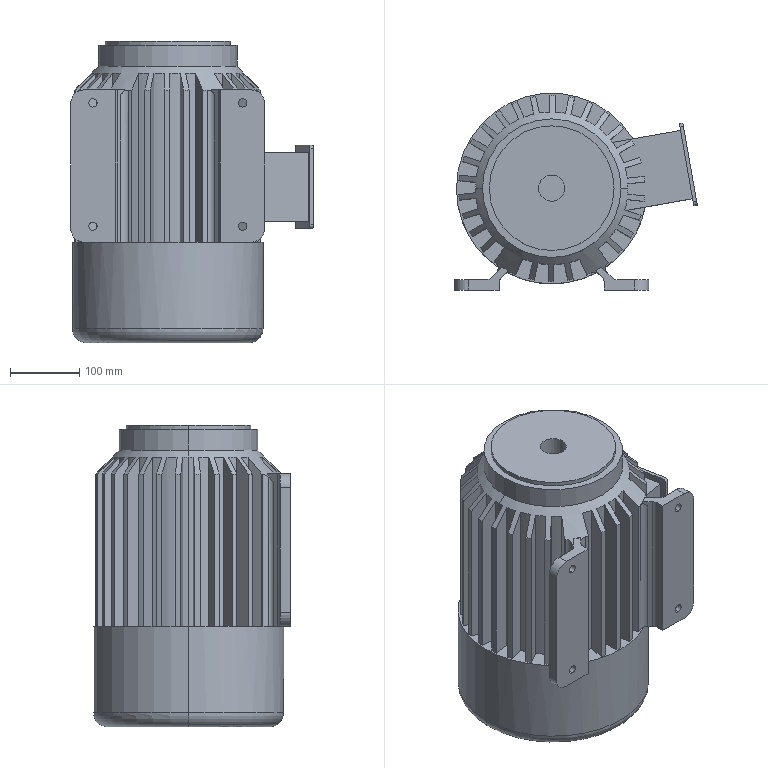Part | SolidWorks | features ICE 6, Fillet 2, Revolution 1 | 1 solid | 202 faces | box 350 x 284.5 x 435 mm | volume 22165719 mm3 | cylinder 102 | plane 96 | torus 2 | cone 2 | commonest cylinder face diameters 269 x36 220 x33 20 x9 12 x8 10 x4 40 x4